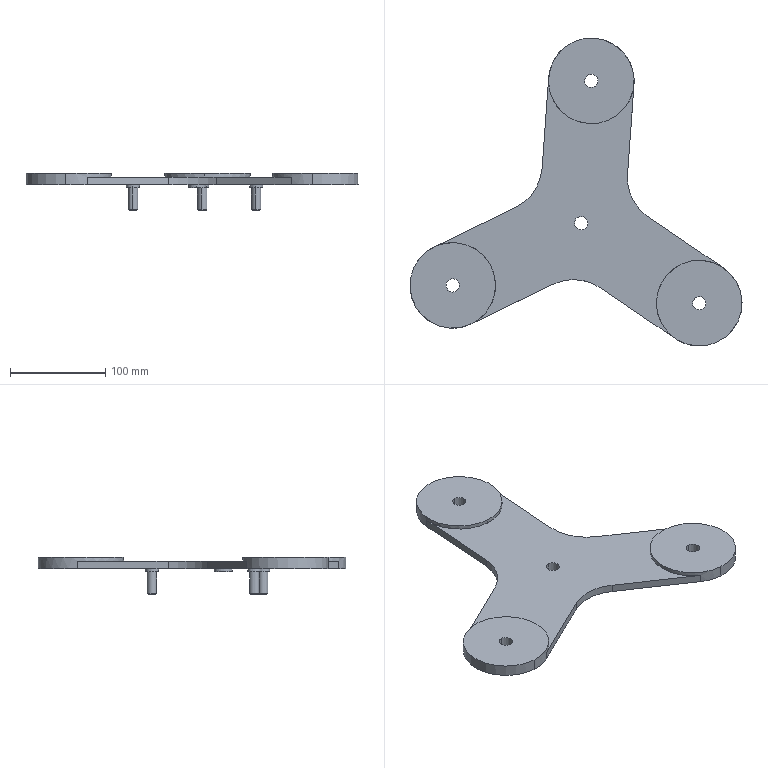Part | SolidWorks | features BaseBody 1 | 1 solid | 55 faces | box 349.137 x 323.748 x 39 mm | volume 452459 mm3 | cylinder 31 | plane 18 | cone 6 | commonest cylinder face diameters 14 x14 10 x6 90 x6 100 x3 19 x2